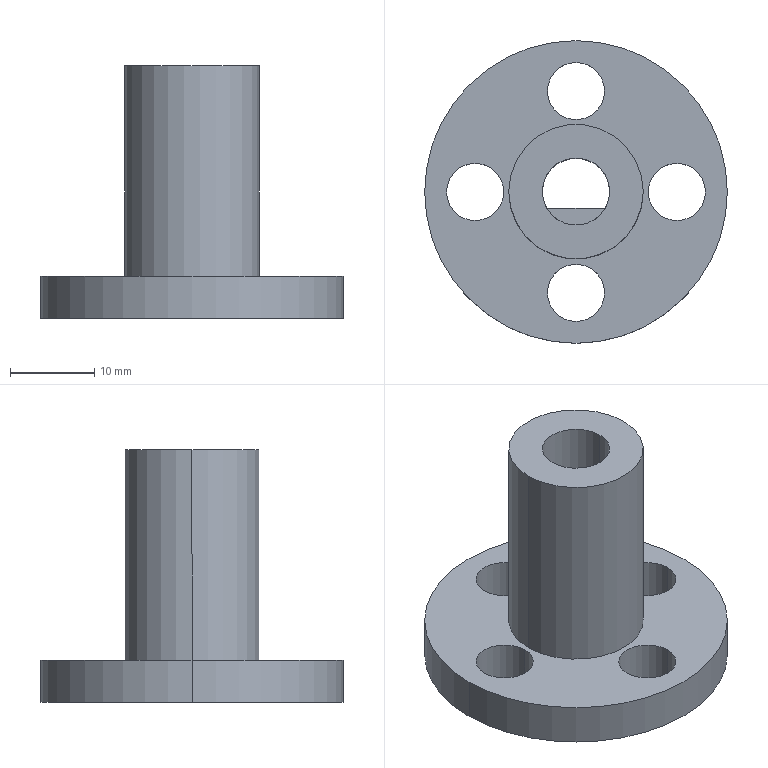Part | SolidWorks | features BaseBody 1 | 1 solid | 19 faces | box 36 x 36 x 30 mm | volume 8127 mm3 | cylinder 14 | plane 5 | commonest cylinder face diameters 6.8 x8 8 x2 16 x2 36 x2
STEP:
#1=CARTESIAN_POINT('',(3.4,12.,5.));
#2=VERTEX_POINT('',#1);
#3=CARTESIAN_POINT('',(3.4,12.,0.));
#4=VERTEX_POINT('',#3);
#5=CARTESIAN_POINT('',(3.4,12.,0.));
#6=DIRECTION('',(0.,0.,-1.));
#7=VECTOR('',#6,1000.);
#8=LINE('',#5,#7);
#9=EDGE_CURVE('',#2,#4,#8,.T.);
#10=ORIENTED_EDGE('',*,*,#9,.F.);
#11=CARTESIAN_POINT('',(-3.4,12.,5.));
#12=VERTEX_POINT('',#11);
#13=CARTESIAN_POINT('',(0.,12.,5.));
#14=DIRECTION('',(0.,0.,1.));
#15=DIRECTION('',(1.,0.,0.));
#16=AXIS2_PLACEMENT_3D('',#13,#14,#15);
#17=CIRCLE('',#16,3.4);
#18=EDGE_CURVE('',#2,#12,#17,.T.);
#19=ORIENTED_EDGE('',*,*,#18,.T.);
#20=CARTESIAN_POINT('',(-3.4,12.,0.));
#21=VERTEX_POINT('',#20);
#22=CARTESIAN_POINT('',(-3.4,12.,0.));
#23=DIRECTION('',(0.,0.,-1.));
#24=VECTOR('',#23,1000.);
#25=LINE('',#22,#24);
#26=EDGE_CURVE('',#12,#21,#25,.T.);
#27=ORIENTED_EDGE('',*,*,#26,.T.);
#28=CARTESIAN_POINT('',(0.,12.,0.));
#29=DIRECTION('',(0.,0.,-1.));
#30=DIRECTION('',(-1.,0.,0.));
#31=AXIS2_PLACEMENT_3D('',#28,#29,#30);
#32=CIRCLE('',#31,3.4);
#33=EDGE_CURVE('',#21,#4,#32,.T.);
#34=ORIENTED_EDGE('',*,*,#33,.T.);
#35=EDGE_LOOP('',(#10,#19,#27,#34));
#36=FACE_OUTER_BOUND('',#35,.T.);
#37=CARTESIAN_POINT('',(0.,12.,0.));
#38=DIRECTION('',(0.,0.,-1.));
#39=DIRECTION('',(-1.,0.,0.));
#40=AXIS2_PLACEMENT_3D('',#37,#38,#39);
#41=CYLINDRICAL_SURFACE('',#40,3.4);
#42=ADVANCED_FACE('',(#36),#41,.F.);
#43=CARTESIAN_POINT('',(15.4,0.,5.));
#44=VERTEX_POINT('',#43);
#45=CARTESIAN_POINT('',(15.4,0.,0.));
#46=VERTEX_POINT('',#45);
#47=CARTESIAN_POINT('',(15.4,0.,0.));
#48=DIRECTION('',(0.,0.,-1.));
#49=VECTOR('',#48,1000.);
#50=LINE('',#47,#49);
#51=EDGE_CURVE('',#44,#46,#50,.T.);
#52=ORIENTED_EDGE('',*,*,#51,.F.);
#53=CARTESIAN_POINT('',(8.6,0.,5.));
#54=VERTEX_POINT('',#53);
#55=CARTESIAN_POINT('',(12.,0.,5.));
#56=DIRECTION('',(0.,0.,1.));
#57=DIRECTION('',(1.,0.,0.));
#58=AXIS2_PLACEMENT_3D('',#55,#56,#57);
#59=CIRCLE('',#58,3.4);
#60=EDGE_CURVE('',#44,#54,#59,.T.);
#61=ORIENTED_EDGE('',*,*,#60,.T.);
#62=CARTESIAN_POINT('',(8.6,0.,0.));
#63=VERTEX_POINT('',#62);
#64=CARTESIAN_POINT('',(8.6,0.,0.));
#65=DIRECTION('',(0.,0.,-1.));
#66=VECTOR('',#65,1000.);
#67=LINE('',#64,#66);
#68=EDGE_CURVE('',#54,#63,#67,.T.);
#69=ORIENTED_EDGE('',*,*,#68,.T.);
#70=CARTESIAN_POINT('',(12.,0.,0.));
#71=DIRECTION('',(0.,0.,-1.));
#72=DIRECTION('',(-1.,0.,0.));
#73=AXIS2_PLACEMENT_3D('',#70,#71,#72);
#74=CIRCLE('',#73,3.4);
#75=EDGE_CURVE('',#63,#46,#74,.T.);
#76=ORIENTED_EDGE('',*,*,#75,.T.);
#77=EDGE_LOOP('',(#52,#61,#69,#76));
#78=FACE_OUTER_BOUND('',#77,.T.);
#79=CARTESIAN_POINT('',(12.,0.,0.));
#80=DIRECTION('',(0.,0.,-1.));
#81=DIRECTION('',(-1.,0.,0.));
#82=AXIS2_PLACEMENT_3D('',#79,#80,#81);
#83=CYLINDRICAL_SURFACE('',#82,3.4);
#84=ADVANCED_FACE('',(#78),#83,.F.);
#85=CARTESIAN_POINT('',(3.4,-12.,5.));
#86=VERTEX_POINT('',#85);
#87=CARTESIAN_POINT('',(3.4,-12.,0.));
#88=VERTEX_POINT('',#87);
#89=CARTESIAN_POINT('',(3.4,-12.,0.));
#90=DIRECTION('',(0.,0.,-1.));
#91=VECTOR('',#90,1000.);
#92=LINE('',#89,#91);
#93=EDGE_CURVE('',#86,#88,#92,.T.);
#94=ORIENTED_EDGE('',*,*,#93,.F.);
#95=CARTESIAN_POINT('',(-3.4,-12.,5.));
#96=VERTEX_POINT('',#95);
#97=CARTESIAN_POINT('',(0.,-12.,5.));
#98=DIRECTION('',(0.,0.,1.));
#99=DIRECTION('',(1.,0.,0.));
#100=AXIS2_PLACEMENT_3D('',#97,#98,#99);
#101=CIRCLE('',#100,3.4);
#102=EDGE_CURVE('',#86,#96,#101,.T.);
#103=ORIENTED_EDGE('',*,*,#102,.T.);
#104=CARTESIAN_POINT('',(-3.4,-12.,0.));
#105=VERTEX_POINT('',#104);
#106=CARTESIAN_POINT('',(-3.4,-12.,0.));
#107=DIRECTION('',(0.,0.,-1.));
#108=VECTOR('',#107,1000.);
#109=LINE('',#106,#108);
#110=EDGE_CURVE('',#96,#105,#109,.T.);
#111=ORIENTED_EDGE('',*,*,#110,.T.);
#112=CARTESIAN_POINT('',(0.,-12.,0.));
#113=DIRECTION('',(0.,0.,-1.));
#114=DIRECTION('',(-1.,0.,0.));
#115=AXIS2_PLACEMENT_3D('',#112,#113,#114);
#116=CIRCLE('',#115,3.4);
#117=EDGE_CURVE('',#105,#88,#116,.T.);
#118=ORIENTED_EDGE('',*,*,#117,.T.);
#119=EDGE_LOOP('',(#94,#103,#111,#118));
#120=FACE_OUTER_BOUND('',#119,.T.);
#121=CARTESIAN_POINT('',(0.,-12.,0.));
#122=DIRECTION('',(0.,0.,-1.));
#123=DIRECTION('',(-1.,0.,0.));
#124=AXIS2_PLACEMENT_3D('',#121,#122,#123);
#125=CYLINDRICAL_SURFACE('',#124,3.4);
#126=ADVANCED_FACE('',(#120),#125,.F.);
#127=CARTESIAN_POINT('',(-8.6,0.,5.));
#128=VERTEX_POINT('',#127);
#129=CARTESIAN_POINT('',(-8.6,0.,0.));
#130=VERTEX_POINT('',#129);
#131=CARTESIAN_POINT('',(-8.6,0.,0.));
#132=DIRECTION('',(0.,0.,-1.));
#133=VECTOR('',#132,1000.);
#134=LINE('',#131,#133);
#135=EDGE_CURVE('',#128,#130,#134,.T.);
#136=ORIENTED_EDGE('',*,*,#135,.F.);
#137=CARTESIAN_POINT('',(-15.4,0.,5.));
#138=VERTEX_POINT('',#137);
#139=CARTESIAN_POINT('',(-12.,0.,5.));
#140=DIRECTION('',(0.,0.,1.));
#141=DIRECTION('',(1.,0.,0.));
#142=AXIS2_PLACEMENT_3D('',#139,#140,#141);
#143=CIRCLE('',#142,3.4);
#144=EDGE_CURVE('',#128,#138,#143,.T.);
#145=ORIENTED_EDGE('',*,*,#144,.T.);
#146=CARTESIAN_POINT('',(-15.4,0.,0.));
#147=VERTEX_POINT('',#146);
#148=CARTESIAN_POINT('',(-15.4,0.,0.));
#149=DIRECTION('',(0.,0.,-1.));
#150=VECTOR('',#149,1000.);
#151=LINE('',#148,#150);
#152=EDGE_CURVE('',#138,#147,#151,.T.);
#153=ORIENTED_EDGE('',*,*,#152,.T.);
#154=CARTESIAN_POINT('',(-12.,0.,0.));
#155=DIRECTION('',(0.,0.,-1.));
#156=DIRECTION('',(-1.,0.,0.));
#157=AXIS2_PLACEMENT_3D('',#154,#155,#156);
#158=CIRCLE('',#157,3.4);
#159=EDGE_CURVE('',#147,#130,#158,.T.);
#160=ORIENTED_EDGE('',*,*,#159,.T.);
#161=EDGE_LOOP('',(#136,#145,#153,#160));
#162=FACE_OUTER_BOUND('',#161,.T.);
#163=CARTESIAN_POINT('',(-12.,0.,0.));
#164=DIRECTION('',(0.,0.,-1.));
#165=DIRECTION('',(-1.,0.,0.));
#166=AXIS2_PLACEMENT_3D('',#163,#164,#165);
#167=CYLINDRICAL_SURFACE('',#166,3.4);
#168=ADVANCED_FACE('',(#162),#167,.F.);
#169=CARTESIAN_POINT('',(-3.464,-2.,0.));
#170=VERTEX_POINT('',#169);
#171=CARTESIAN_POINT('',(3.464,-2.,0.));
#172=VERTEX_POINT('',#171);
#173=CARTESIAN_POINT('',(3.464,-2.,0.));
#174=DIRECTION('',(1.,0.,0.));
#175=VECTOR('',#174,1000.);
#176=LINE('',#173,#175);
#177=EDGE_CURVE('',#170,#172,#176,.T.);
#178=ORIENTED_EDGE('',*,*,#177,.F.);
#179=CARTESIAN_POINT('',(-3.464,-2.,25.));
#180=VERTEX_POINT('',#179);
#181=CARTESIAN_POINT('',(-3.464,-2.,25.));
#182=DIRECTION('',(0.,0.,-1.));
#183=VECTOR('',#182,1000.);
#184=LINE('',#181,#183);
#185=EDGE_CURVE('',#180,#170,#184,.T.);
#186=ORIENTED_EDGE('',*,*,#185,.F.);
#187=CARTESIAN_POINT('',(3.464,-2.,25.));
#188=VERTEX_POINT('',#187);
#189=CARTESIAN_POINT('',(3.464,-2.,25.));
#190=DIRECTION('',(1.,0.,0.));
#191=VECTOR('',#190,1000.);
#192=LINE('',#189,#191);
#193=EDGE_CURVE('',#180,#188,#192,.T.);
#194=ORIENTED_EDGE('',*,*,#193,.T.);
#195=CARTESIAN_POINT('',(3.464,-2.,25.));
#196=DIRECTION('',(0.,0.,-1.));
#197=VECTOR('',#196,1000.);
#198=LINE('',#195,#197);
#199=EDGE_CURVE('',#188,#172,#198,.T.);
#200=ORIENTED_EDGE('',*,*,#199,.T.);
#201=EDGE_LOOP('',(#178,#186,#194,#200));
#202=FACE_OUTER_BOUND('',#201,.T.);
#203=CARTESIAN_POINT('',(3.464,-2.,25.));
#204=DIRECTION('',(0.,1.,0.));
#205=DIRECTION('',(1.,0.,0.));
#206=AXIS2_PLACEMENT_3D('',#203,#204,#205);
#207=PLANE('',#206);
#208=ADVANCED_FACE('',(#202),#207,.T.);
#209=CARTESIAN_POINT('',(0.,0.,25.));
#210=DIRECTION('',(0.,0.,-1.));
#211=DIRECTION('',(-1.,0.,0.));
#212=AXIS2_PLACEMENT_3D('',#209,#210,#211);
#213=CIRCLE('',#212,4.);
#214=EDGE_CURVE('',#188,#180,#213,.T.);
#215=ORIENTED_EDGE('',*,*,#214,.F.);
#216=ORIENTED_EDGE('',*,*,#193,.F.);
#217=EDGE_LOOP('',(#215,#216));
#218=FACE_OUTER_BOUND('',#217,.T.);
#219=CARTESIAN_POINT('',(0.,0.,25.));
#220=DIRECTION('',(0.,0.,-1.));
#221=DIRECTION('',(0.,-1.,0.));
#222=AXIS2_PLACEMENT_3D('',#219,#220,#221);
#223=PLANE('',#222);
#224=ADVANCED_FACE('',(#218),#223,.F.);
#225=CARTESIAN_POINT('',(-4.,0.,30.));
#226=VERTEX_POINT('',#225);
#227=CARTESIAN_POINT('',(4.,0.,30.));
#228=VERTEX_POINT('',#227);
#229=CARTESIAN_POINT('',(0.,0.,30.));
#230=DIRECTION('',(0.,0.,1.));
#231=DIRECTION('',(1.,0.,0.));
#232=AXIS2_PLACEMENT_3D('',#229,#230,#231);
#233=CIRCLE('',#232,4.);
#234=EDGE_CURVE('',#226,#228,#233,.T.);
#235=ORIENTED_EDGE('',*,*,#234,.F.);
#236=CARTESIAN_POINT('',(0.,0.,30.));
#237=DIRECTION('',(0.,0.,1.));
#238=DIRECTION('',(1.,0.,0.));
#239=AXIS2_PLACEMENT_3D('',#236,#237,#238);
#240=CIRCLE('',#239,4.);
#241=EDGE_CURVE('',#228,#226,#240,.T.);
#242=ORIENTED_EDGE('',*,*,#241,.F.);
#243=EDGE_LOOP('',(#235,#242));
#244=FACE_BOUND('',#243,.T.);
#245=CARTESIAN_POINT('',(-8.,0.,30.));
#246=VERTEX_POINT('',#245);
#247=CARTESIAN_POINT('',(8.,0.,30.));
#248=VERTEX_POINT('',#247);
#249=CARTESIAN_POINT('',(0.,0.,30.));
#250=DIRECTION('',(0.,0.,1.));
#251=DIRECTION('',(1.,0.,0.));
#252=AXIS2_PLACEMENT_3D('',#249,#250,#251);
#253=CIRCLE('',#252,8.);
#254=EDGE_CURVE('',#246,#248,#253,.T.);
#255=ORIENTED_EDGE('',*,*,#254,.T.);
#256=CARTESIAN_POINT('',(0.,0.,30.));
#257=DIRECTION('',(0.,0.,1.));
#258=DIRECTION('',(1.,0.,0.));
#259=AXIS2_PLACEMENT_3D('',#256,#257,#258);
#260=CIRCLE('',#259,8.);
#261=EDGE_CURVE('',#248,#246,#260,.T.);
#262=ORIENTED_EDGE('',*,*,#261,.T.);
#263=EDGE_LOOP('',(#255,#262));
#264=FACE_OUTER_BOUND('',#263,.T.);
#265=CARTESIAN_POINT('',(0.,0.,30.));
#266=DIRECTION('',(0.,0.,1.));
#267=DIRECTION('',(1.,0.,0.));
#268=AXIS2_PLACEMENT_3D('',#265,#266,#267);
#269=PLANE('',#268);
#270=ADVANCED_FACE('',(#244,#264),#269,.T.);
#271=CARTESIAN_POINT('',(8.,0.,5.));
#272=VERTEX_POINT('',#271);
#273=CARTESIAN_POINT('',(8.,0.,30.));
#274=DIRECTION('',(0.,0.,-1.));
#275=VECTOR('',#274,1000.);
#276=LINE('',#273,#275);
#277=EDGE_CURVE('',#248,#272,#276,.T.);
#278=ORIENTED_EDGE('',*,*,#277,.F.);
#279=ORIENTED_EDGE('',*,*,#254,.F.);
#280=CARTESIAN_POINT('',(-8.,0.,5.));
#281=VERTEX_POINT('',#280);
#282=CARTESIAN_POINT('',(-8.,0.,30.));
#283=DIRECTION('',(0.,0.,-1.));
#284=VECTOR('',#283,1000.);
#285=LINE('',#282,#284);
#286=EDGE_CURVE('',#246,#281,#285,.T.);
#287=ORIENTED_EDGE('',*,*,#286,.T.);
#288=CARTESIAN_POINT('',(0.,0.,5.));
#289=DIRECTION('',(0.,0.,1.));
#290=DIRECTION('',(1.,0.,0.));
#291=AXIS2_PLACEMENT_3D('',#288,#289,#290);
#292=CIRCLE('',#291,8.);
#293=EDGE_CURVE('',#281,#272,#292,.T.);
#294=ORIENTED_EDGE('',*,*,#293,.T.);
#295=EDGE_LOOP('',(#278,#279,#287,#294));
#296=FACE_OUTER_BOUND('',#295,.T.);
#297=CARTESIAN_POINT('',(0.,0.,30.));
#298=DIRECTION('',(0.,0.,-1.));
#299=DIRECTION('',(-1.,0.,0.));
#300=AXIS2_PLACEMENT_3D('',#297,#298,#299);
#301=CYLINDRICAL_SURFACE('',#300,8.);
#302=ADVANCED_FACE('',(#296),#301,.T.);
#303=CARTESIAN_POINT('',(4.,0.,0.));
#304=VERTEX_POINT('',#303);
#305=CARTESIAN_POINT('',(4.,0.,30.));
#306=DIRECTION('',(0.,0.,-1.));
#307=VECTOR('',#306,1000.);
#308=LINE('',#305,#307);
#309=EDGE_CURVE('',#228,#304,#308,.T.);
#310=ORIENTED_EDGE('',*,*,#309,.F.);
#311=ORIENTED_EDGE('',*,*,#241,.T.);
#312=CARTESIAN_POINT('',(-4.,0.,0.));
#313=VERTEX_POINT('',#312);
#314=CARTESIAN_POINT('',(-4.,0.,30.));
#315=DIRECTION('',(0.,0.,-1.));
#316=VECTOR('',#315,1000.);
#317=LINE('',#314,#316);
#318=EDGE_CURVE('',#226,#313,#317,.T.);
#319=ORIENTED_EDGE('',*,*,#318,.T.);
#320=CARTESIAN_POINT('',(0.,0.,0.));
#321=DIRECTION('',(0.,0.,1.));
#322=DIRECTION('',(1.,0.,0.));
#323=AXIS2_PLACEMENT_3D('',#320,#321,#322);
#324=CIRCLE('',#323,4.);
#325=EDGE_CURVE('',#304,#313,#324,.T.);
#326=ORIENTED_EDGE('',*,*,#325,.F.);
#327=EDGE_LOOP('',(#310,#311,#319,#326));
#328=FACE_OUTER_BOUND('',#327,.T.);
#329=CARTESIAN_POINT('',(0.,0.,30.));
#330=DIRECTION('',(0.,0.,-1.));
#331=DIRECTION('',(-1.,0.,0.));
#332=AXIS2_PLACEMENT_3D('',#329,#330,#331);
#333=CYLINDRICAL_SURFACE('',#332,4.);
#334=ADVANCED_FACE('',(#328),#333,.F.);
#335=ORIENTED_EDGE('',*,*,#177,.T.);
#336=CARTESIAN_POINT('',(0.,0.,0.));
#337=DIRECTION('',(0.,0.,1.));
#338=DIRECTION('',(1.,0.,0.));
#339=AXIS2_PLACEMENT_3D('',#336,#337,#338);
#340=CIRCLE('',#339,4.);
#341=EDGE_CURVE('',#172,#304,#340,.T.);
#342=ORIENTED_EDGE('',*,*,#341,.T.);
#343=ORIENTED_EDGE('',*,*,#325,.T.);
#344=CARTESIAN_POINT('',(0.,0.,0.));
#345=DIRECTION('',(0.,0.,1.));
#346=DIRECTION('',(1.,0.,0.));
#347=AXIS2_PLACEMENT_3D('',#344,#345,#346);
#348=CIRCLE('',#347,4.);
#349=EDGE_CURVE('',#313,#170,#348,.T.);
#350=ORIENTED_EDGE('',*,*,#349,.T.);
#351=EDGE_LOOP('',(#335,#342,#343,#350));
#352=FACE_BOUND('',#351,.T.);
#353=ORIENTED_EDGE('',*,*,#159,.F.);
#354=CARTESIAN_POINT('',(-12.,0.,0.));
#355=DIRECTION('',(0.,0.,-1.));
#356=DIRECTION('',(-1.,0.,0.));
#357=AXIS2_PLACEMENT_3D('',#354,#355,#356);
#358=CIRCLE('',#357,3.4);
#359=EDGE_CURVE('',#130,#147,#358,.T.);
#360=ORIENTED_EDGE('',*,*,#359,.F.);
#361=EDGE_LOOP('',(#353,#360));
#362=FACE_BOUND('',#361,.T.);
#363=ORIENTED_EDGE('',*,*,#117,.F.);
#364=CARTESIAN_POINT('',(0.,-12.,0.));
#365=DIRECTION('',(0.,0.,-1.));
#366=DIRECTION('',(-1.,0.,0.));
#367=AXIS2_PLACEMENT_3D('',#364,#365,#366);
#368=CIRCLE('',#367,3.4);
#369=EDGE_CURVE('',#88,#105,#368,.T.);
#370=ORIENTED_EDGE('',*,*,#369,.F.);
#371=EDGE_LOOP('',(#363,#370));
#372=FACE_BOUND('',#371,.T.);
#373=ORIENTED_EDGE('',*,*,#75,.F.);
#374=CARTESIAN_POINT('',(12.,0.,0.));
#375=DIRECTION('',(0.,0.,-1.));
#376=DIRECTION('',(-1.,0.,0.));
#377=AXIS2_PLACEMENT_3D('',#374,#375,#376);
#378=CIRCLE('',#377,3.4);
#379=EDGE_CURVE('',#46,#63,#378,.T.);
#380=ORIENTED_EDGE('',*,*,#379,.F.);
#381=EDGE_LOOP('',(#373,#380));
#382=FACE_BOUND('',#381,.T.);
#383=ORIENTED_EDGE('',*,*,#33,.F.);
#384=CARTESIAN_POINT('',(0.,12.,0.));
#385=DIRECTION('',(0.,0.,-1.));
#386=DIRECTION('',(-1.,0.,0.));
#387=AXIS2_PLACEMENT_3D('',#384,#385,#386);
#388=CIRCLE('',#387,3.4);
#389=EDGE_CURVE('',#4,#21,#388,.T.);
#390=ORIENTED_EDGE('',*,*,#389,.F.);
#391=EDGE_LOOP('',(#383,#390));
#392=FACE_BOUND('',#391,.T.);
#393=CARTESIAN_POINT('',(-18.,0.,0.));
#394=VERTEX_POINT('',#393);
#395=CARTESIAN_POINT('',(18.,0.,0.));
#396=VERTEX_POINT('',#395);
#397=CARTESIAN_POINT('',(0.,0.,0.));
#398=DIRECTION('',(0.,0.,1.));
#399=DIRECTION('',(1.,0.,0.));
#400=AXIS2_PLACEMENT_3D('',#397,#398,#399);
#401=CIRCLE('',#400,18.);
#402=EDGE_CURVE('',#394,#396,#401,.T.);
#403=ORIENTED_EDGE('',*,*,#402,.F.);
#404=CARTESIAN_POINT('',(0.,0.,0.));
#405=DIRECTION('',(0.,0.,1.));
#406=DIRECTION('',(1.,0.,0.));
#407=AXIS2_PLACEMENT_3D('',#404,#405,#406);
#408=CIRCLE('',#407,18.);
#409=EDGE_CURVE('',#396,#394,#408,.T.);
#410=ORIENTED_EDGE('',*,*,#409,.F.);
#411=EDGE_LOOP('',(#403,#410));
#412=FACE_OUTER_BOUND('',#411,.T.);
#413=CARTESIAN_POINT('',(0.,0.,0.));
#414=DIRECTION('',(0.,0.,1.));
#415=DIRECTION('',(1.,0.,0.));
#416=AXIS2_PLACEMENT_3D('',#413,#414,#415);
#417=PLANE('',#416);
#418=ADVANCED_FACE('',(#352,#362,#372,#382,#392,#412),#417,.F.);
#419=ORIENTED_EDGE('',*,*,#293,.F.);
#420=CARTESIAN_POINT('',(0.,0.,5.));
#421=DIRECTION('',(0.,0.,1.));
#422=DIRECTION('',(1.,0.,0.));
#423=AXIS2_PLACEMENT_3D('',#420,#421,#422);
#424=CIRCLE('',#423,8.);
#425=EDGE_CURVE('',#272,#281,#424,.T.);
#426=ORIENTED_EDGE('',*,*,#425,.F.);
#427=EDGE_LOOP('',(#419,#426));
#428=FACE_BOUND('',#427,.T.);
#429=CARTESIAN_POINT('',(-12.,0.,5.));
#430=DIRECTION('',(0.,0.,1.));
#431=DIRECTION('',(1.,0.,0.));
#432=AXIS2_PLACEMENT_3D('',#429,#430,#431);
#433=CIRCLE('',#432,3.4);
#434=EDGE_CURVE('',#138,#128,#433,.T.);
#435=ORIENTED_EDGE('',*,*,#434,.F.);
#436=ORIENTED_EDGE('',*,*,#144,.F.);
#437=EDGE_LOOP('',(#435,#436));
#438=FACE_BOUND('',#437,.T.);
#439=CARTESIAN_POINT('',(0.,-12.,5.));
#440=DIRECTION('',(0.,0.,1.));
#441=DIRECTION('',(1.,0.,0.));
#442=AXIS2_PLACEMENT_3D('',#439,#440,#441);
#443=CIRCLE('',#442,3.4);
#444=EDGE_CURVE('',#96,#86,#443,.T.);
#445=ORIENTED_EDGE('',*,*,#444,.F.);
#446=ORIENTED_EDGE('',*,*,#102,.F.);
#447=EDGE_LOOP('',(#445,#446));
#448=FACE_BOUND('',#447,.T.);
#449=CARTESIAN_POINT('',(12.,0.,5.));
#450=DIRECTION('',(0.,0.,1.));
#451=DIRECTION('',(1.,0.,0.));
#452=AXIS2_PLACEMENT_3D('',#449,#450,#451);
#453=CIRCLE('',#452,3.4);
#454=EDGE_CURVE('',#54,#44,#453,.T.);
#455=ORIENTED_EDGE('',*,*,#454,.F.);
#456=ORIENTED_EDGE('',*,*,#60,.F.);
#457=EDGE_LOOP('',(#455,#456));
#458=FACE_BOUND('',#457,.T.);
#459=CARTESIAN_POINT('',(0.,12.,5.));
#460=DIRECTION('',(0.,0.,1.));
#461=DIRECTION('',(1.,0.,0.));
#462=AXIS2_PLACEMENT_3D('',#459,#460,#461);
#463=CIRCLE('',#462,3.4);
#464=EDGE_CURVE('',#12,#2,#463,.T.);
#465=ORIENTED_EDGE('',*,*,#464,.F.);
#466=ORIENTED_EDGE('',*,*,#18,.F.);
#467=EDGE_LOOP('',(#465,#466));
#468=FACE_BOUND('',#467,.T.);
#469=CARTESIAN_POINT('',(-18.,0.,5.));
#470=VERTEX_POINT('',#469);
#471=CARTESIAN_POINT('',(18.,0.,5.));
#472=VERTEX_POINT('',#471);
#473=CARTESIAN_POINT('',(0.,0.,5.));
#474=DIRECTION('',(0.,0.,1.));
#475=DIRECTION('',(1.,0.,0.));
#476=AXIS2_PLACEMENT_3D('',#473,#474,#475);
#477=CIRCLE('',#476,18.);
#478=EDGE_CURVE('',#470,#472,#477,.T.);
#479=ORIENTED_EDGE('',*,*,#478,.T.);
#480=CARTESIAN_POINT('',(0.,0.,5.));
#481=DIRECTION('',(0.,0.,1.));
#482=DIRECTION('',(1.,0.,0.));
#483=AXIS2_PLACEMENT_3D('',#480,#481,#482);
#484=CIRCLE('',#483,18.);
#485=EDGE_CURVE('',#472,#470,#484,.T.);
#486=ORIENTED_EDGE('',*,*,#485,.T.);
#487=EDGE_LOOP('',(#479,#486));
#488=FACE_OUTER_BOUND('',#487,.T.);
#489=CARTESIAN_POINT('',(0.,0.,5.));
#490=DIRECTION('',(0.,0.,1.));
#491=DIRECTION('',(1.,0.,0.));
#492=AXIS2_PLACEMENT_3D('',#489,#490,#491);
#493=PLANE('',#492);
#494=ADVANCED_FACE('',(#428,#438,#448,#458,#468,#488),#493,.T.);
#495=CARTESIAN_POINT('',(18.,0.,5.));
#496=DIRECTION('',(0.,0.,-1.));
#497=VECTOR('',#496,1000.);
#498=LINE('',#495,#497);
#499=EDGE_CURVE('',#472,#396,#498,.T.);
#500=ORIENTED_EDGE('',*,*,#499,.F.);
#501=ORIENTED_EDGE('',*,*,#478,.F.);
#502=CARTESIAN_POINT('',(-18.,0.,5.));
#503=DIRECTION('',(0.,0.,-1.));
#504=VECTOR('',#503,1000.);
#505=LINE('',#502,#504);
#506=EDGE_CURVE('',#470,#394,#505,.T.);
#507=ORIENTED_EDGE('',*,*,#506,.T.);
#508=ORIENTED_EDGE('',*,*,#402,.T.);
#509=EDGE_LOOP('',(#500,#501,#507,#508));
#510=FACE_OUTER_BOUND('',#509,.T.);
#511=CARTESIAN_POINT('',(0.,0.,5.));
#512=DIRECTION('',(0.,0.,-1.));
#513=DIRECTION('',(-1.,0.,0.));
#514=AXIS2_PLACEMENT_3D('',#511,#512,#513);
#515=CYLINDRICAL_SURFACE('',#514,18.);
#516=ADVANCED_FACE('',(#510),#515,.T.);
#517=ORIENTED_EDGE('',*,*,#485,.F.);
#518=ORIENTED_EDGE('',*,*,#499,.T.);
#519=ORIENTED_EDGE('',*,*,#409,.T.);
#520=ORIENTED_EDGE('',*,*,#506,.F.);
#521=EDGE_LOOP('',(#517,#518,#519,#520));
#522=FACE_OUTER_BOUND('',#521,.T.);
#523=CARTESIAN_POINT('',(0.,0.,5.));
#524=DIRECTION('',(0.,0.,-1.));
#525=DIRECTION('',(-1.,0.,0.));
#526=AXIS2_PLACEMENT_3D('',#523,#524,#525);
#527=CYLINDRICAL_SURFACE('',#526,18.);
#528=ADVANCED_FACE('',(#522),#527,.T.);
#529=ORIENTED_EDGE('',*,*,#234,.T.);
#530=ORIENTED_EDGE('',*,*,#309,.T.);
#531=ORIENTED_EDGE('',*,*,#341,.F.);
#532=ORIENTED_EDGE('',*,*,#199,.F.);
#533=ORIENTED_EDGE('',*,*,#214,.T.);
#534=ORIENTED_EDGE('',*,*,#185,.T.);
#535=ORIENTED_EDGE('',*,*,#349,.F.);
#536=ORIENTED_EDGE('',*,*,#318,.F.);
#537=EDGE_LOOP('',(#529,#530,#531,#532,#533,#534,#535,#536));
#538=FACE_OUTER_BOUND('',#537,.T.);
#539=CARTESIAN_POINT('',(0.,0.,30.));
#540=DIRECTION('',(0.,0.,-1.));
#541=DIRECTION('',(-1.,0.,0.));
#542=AXIS2_PLACEMENT_3D('',#539,#540,#541);
#543=CYLINDRICAL_SURFACE('',#542,4.);
#544=ADVANCED_FACE('',(#538),#543,.F.);
#545=ORIENTED_EDGE('',*,*,#261,.F.);
#546=ORIENTED_EDGE('',*,*,#277,.T.);
#547=ORIENTED_EDGE('',*,*,#425,.T.);
#548=ORIENTED_EDGE('',*,*,#286,.F.);
#549=EDGE_LOOP('',(#545,#546,#547,#548));
#550=FACE_OUTER_BOUND('',#549,.T.);
#551=CARTESIAN_POINT('',(0.,0.,30.));
#552=DIRECTION('',(0.,0.,-1.));
#553=DIRECTION('',(-1.,0.,0.));
#554=AXIS2_PLACEMENT_3D('',#551,#552,#553);
#555=CYLINDRICAL_SURFACE('',#554,8.);
#556=ADVANCED_FACE('',(#550),#555,.T.);
#557=ORIENTED_EDGE('',*,*,#434,.T.);
#558=ORIENTED_EDGE('',*,*,#135,.T.);
#559=ORIENTED_EDGE('',*,*,#359,.T.);
#560=ORIENTED_EDGE('',*,*,#152,.F.);
#561=EDGE_LOOP('',(#557,#558,#559,#560));
#562=FACE_OUTER_BOUND('',#561,.T.);
#563=CARTESIAN_POINT('',(-12.,0.,0.));
#564=DIRECTION('',(0.,0.,-1.));
#565=DIRECTION('',(-1.,0.,0.));
#566=AXIS2_PLACEMENT_3D('',#563,#564,#565);
#567=CYLINDRICAL_SURFACE('',#566,3.4);
#568=ADVANCED_FACE('',(#562),#567,.F.);
#569=ORIENTED_EDGE('',*,*,#444,.T.);
#570=ORIENTED_EDGE('',*,*,#93,.T.);
#571=ORIENTED_EDGE('',*,*,#369,.T.);
#572=ORIENTED_EDGE('',*,*,#110,.F.);
#573=EDGE_LOOP('',(#569,#570,#571,#572));
#574=FACE_OUTER_BOUND('',#573,.T.);
#575=CARTESIAN_POINT('',(0.,-12.,0.));
#576=DIRECTION('',(0.,0.,-1.));
#577=DIRECTION('',(-1.,0.,0.));
#578=AXIS2_PLACEMENT_3D('',#575,#576,#577);
#579=CYLINDRICAL_SURFACE('',#578,3.4);
#580=ADVANCED_FACE('',(#574),#579,.F.);
#581=ORIENTED_EDGE('',*,*,#454,.T.);
#582=ORIENTED_EDGE('',*,*,#51,.T.);
#583=ORIENTED_EDGE('',*,*,#379,.T.);
#584=ORIENTED_EDGE('',*,*,#68,.F.);
#585=EDGE_LOOP('',(#581,#582,#583,#584));
#586=FACE_OUTER_BOUND('',#585,.T.);
#587=CARTESIAN_POINT('',(12.,0.,0.));
#588=DIRECTION('',(0.,0.,-1.));
#589=DIRECTION('',(-1.,0.,0.));
#590=AXIS2_PLACEMENT_3D('',#587,#588,#589);
#591=CYLINDRICAL_SURFACE('',#590,3.4);
#592=ADVANCED_FACE('',(#586),#591,.F.);
#593=ORIENTED_EDGE('',*,*,#464,.T.);
#594=ORIENTED_EDGE('',*,*,#9,.T.);
#595=ORIENTED_EDGE('',*,*,#389,.T.);
#596=ORIENTED_EDGE('',*,*,#26,.F.);
#597=EDGE_LOOP('',(#593,#594,#595,#596));
#598=FACE_OUTER_BOUND('',#597,.T.);
#599=CARTESIAN_POINT('',(0.,12.,0.));
#600=DIRECTION('',(0.,0.,-1.));
#601=DIRECTION('',(-1.,0.,0.));
#602=AXIS2_PLACEMENT_3D('',#599,#600,#601);
#603=CYLINDRICAL_SURFACE('',#602,3.4);
#604=ADVANCED_FACE('',(#598),#603,.F.);
#605=CLOSED_SHELL('',(#42,#84,#126,#168,#208,#224,#270,#302,#334,#418,#494,#516,#528,#544,#556,#568,#580,#592,#604));
#606=MANIFOLD_SOLID_BREP('',#605);
#607=CARTESIAN_POINT('',(0.,0.,0.));
#608=DIRECTION('',(0.,0.,1.));
#609=DIRECTION('',(1.,0.,0.));
#610=AXIS2_PLACEMENT_3D('',#607,#608,#609);
#611=(LENGTH_UNIT()NAMED_UNIT(*)SI_UNIT(.MILLI.,.METRE.));
#612=UNCERTAINTY_MEASURE_WITH_UNIT(LENGTH_MEASURE(0.00001),#611,'','');
#613=(NAMED_UNIT(*)PLANE_ANGLE_UNIT()SI_UNIT($,.RADIAN.));
#614=(NAMED_UNIT(*)SI_UNIT($,.STERADIAN.)SOLID_ANGLE_UNIT());
#615=(GEOMETRIC_REPRESENTATION_CONTEXT(3)GLOBAL_UNCERTAINTY_ASSIGNED_CONTEXT((#612))GLOBAL_UNIT_ASSIGNED_CONTEXT((#611,#613,#614))REPRESENTATION_CONTEXT('',''));
#616=ADVANCED_BREP_SHAPE_REPRESENTATION('',(#606,#610),#615);